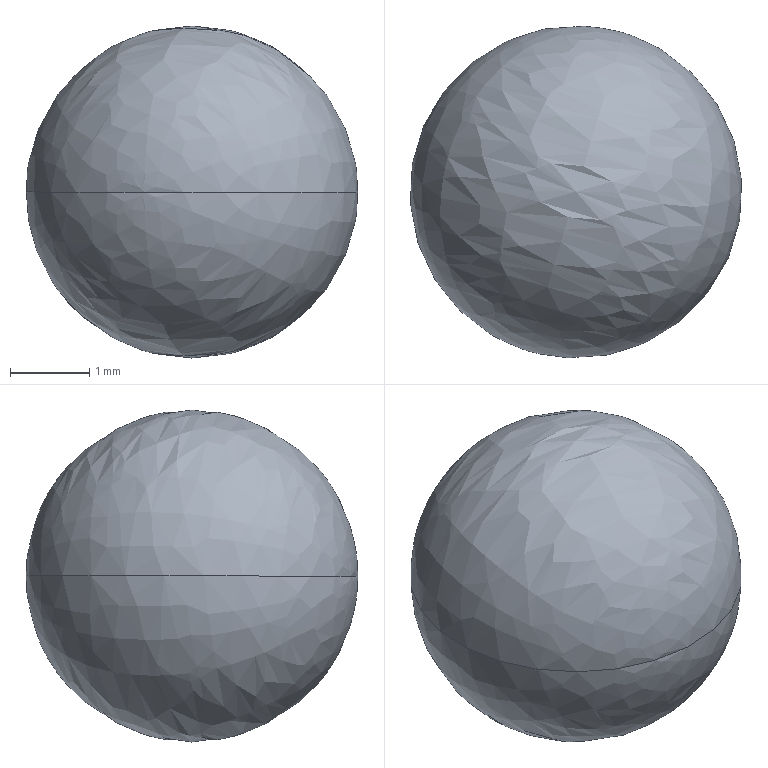Part | SolidWorks | features BaseBody 1 | 1 solid | 2 faces | box 4.2 x 4.2 x 4.2 mm | volume 38.791 mm3 | spline 2